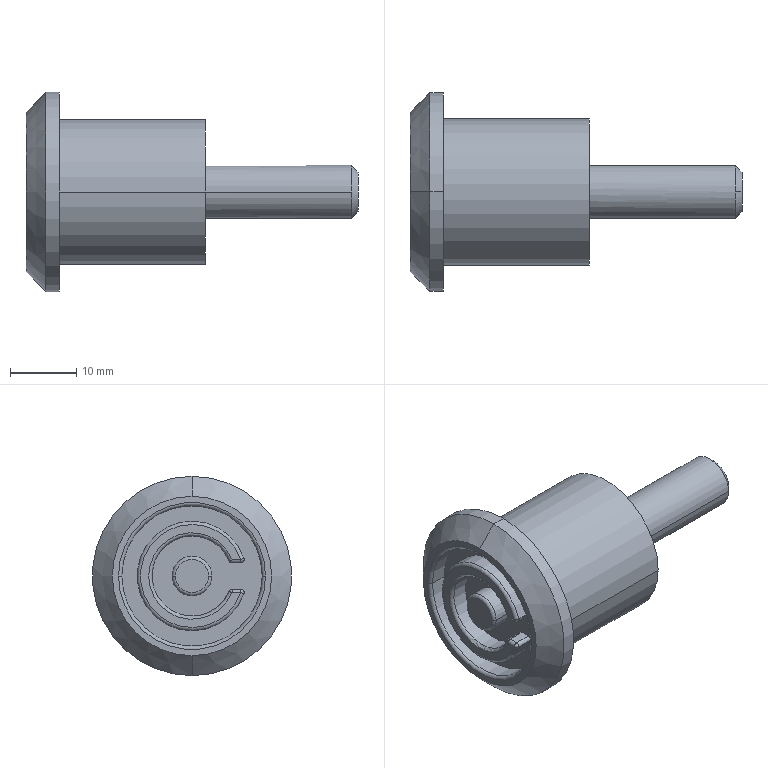Part | STEP file | Cylinder lock | 1 solid | 41 faces | box 50 x 30 x 30 mm | volume 11941 mm3 | cylinder 19 | plane 9 | torus 6 | cone 4 | sphere 3 | commonest cylinder face diameters 1 x7 6 x2 8 x2 21.144 x2 22 x2 30 x2